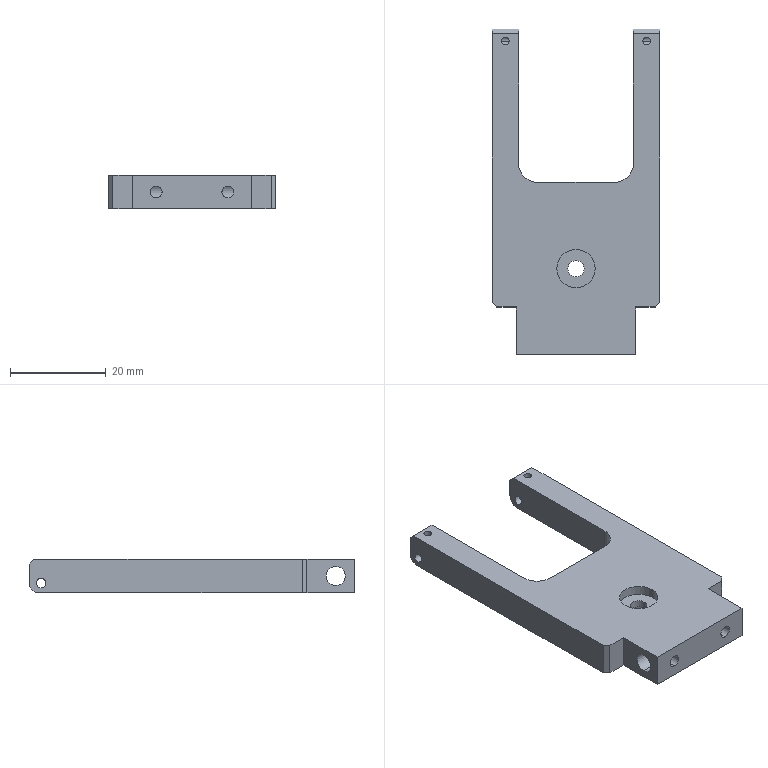Part | SolidWorks | features ICE 4, HoleWzd 3, Fillet 2, Chamfer 1, Extrusion 1 | 1 solid | 44 faces | box 35 x 68 x 7 mm | volume 9996 mm3 | cylinder 24 | plane 20 | commonest cylinder face diameters 1.6 x4 2 x4 2.5 x4 4 x4 8 x4 3.4 x2